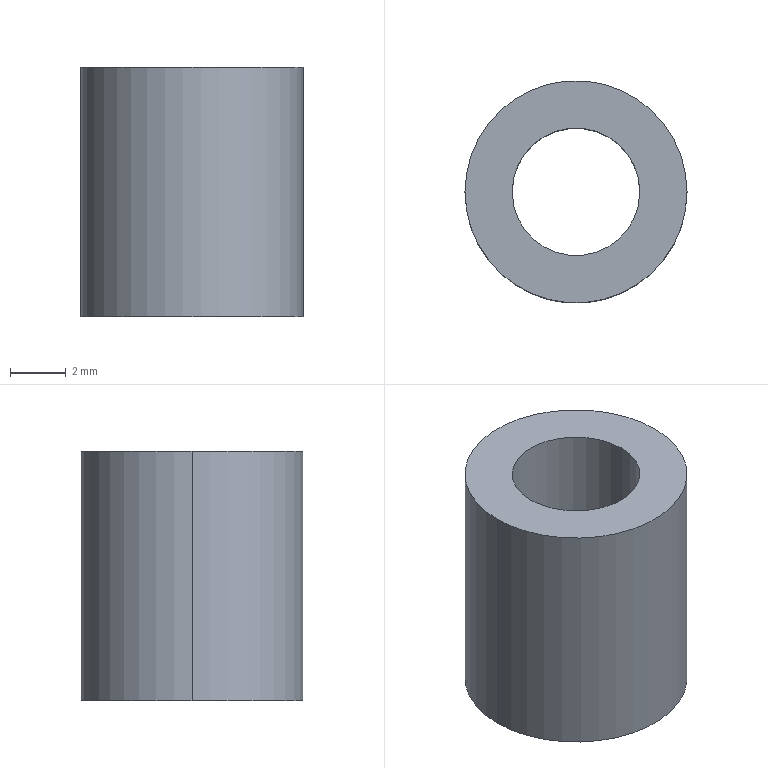Part | SolidWorks | features Extrusion 1 | 1 solid | 6 faces | box 8 x 8 x 9 mm | volume 302.818 mm3 | cylinder 4 | plane 2 | commonest cylinder face diameters 4.6 x2 8 x2
STEP:
#1=CARTESIAN_POINT('',(-2.3,0.,9.));
#2=VERTEX_POINT('',#1);
#3=CARTESIAN_POINT('',(2.3,0.,9.));
#4=VERTEX_POINT('',#3);
#5=CARTESIAN_POINT('',(0.,0.,9.));
#6=DIRECTION('',(0.,0.,1.));
#7=DIRECTION('',(1.,0.,0.));
#8=AXIS2_PLACEMENT_3D('',#5,#6,#7);
#9=CIRCLE('',#8,2.3);
#10=EDGE_CURVE('',#2,#4,#9,.T.);
#11=ORIENTED_EDGE('',*,*,#10,.T.);
#12=CARTESIAN_POINT('',(2.3,0.,0.));
#13=VERTEX_POINT('',#12);
#14=CARTESIAN_POINT('',(2.3,0.,9.));
#15=DIRECTION('',(0.,0.,-1.));
#16=VECTOR('',#15,1000.);
#17=LINE('',#14,#16);
#18=EDGE_CURVE('',#4,#13,#17,.T.);
#19=ORIENTED_EDGE('',*,*,#18,.T.);
#20=CARTESIAN_POINT('',(-2.3,0.,0.));
#21=VERTEX_POINT('',#20);
#22=CARTESIAN_POINT('',(0.,0.,0.));
#23=DIRECTION('',(0.,0.,1.));
#24=DIRECTION('',(1.,0.,0.));
#25=AXIS2_PLACEMENT_3D('',#22,#23,#24);
#26=CIRCLE('',#25,2.3);
#27=EDGE_CURVE('',#21,#13,#26,.T.);
#28=ORIENTED_EDGE('',*,*,#27,.F.);
#29=CARTESIAN_POINT('',(-2.3,0.,9.));
#30=DIRECTION('',(0.,0.,-1.));
#31=VECTOR('',#30,1000.);
#32=LINE('',#29,#31);
#33=EDGE_CURVE('',#2,#21,#32,.T.);
#34=ORIENTED_EDGE('',*,*,#33,.F.);
#35=EDGE_LOOP('',(#11,#19,#28,#34));
#36=FACE_OUTER_BOUND('',#35,.T.);
#37=CARTESIAN_POINT('',(0.,0.,9.));
#38=DIRECTION('',(0.,0.,-1.));
#39=DIRECTION('',(-1.,0.,0.));
#40=AXIS2_PLACEMENT_3D('',#37,#38,#39);
#41=CYLINDRICAL_SURFACE('',#40,2.3);
#42=ADVANCED_FACE('',(#36),#41,.F.);
#43=CARTESIAN_POINT('',(4.,0.,9.));
#44=VERTEX_POINT('',#43);
#45=CARTESIAN_POINT('',(-4.,0.,9.));
#46=VERTEX_POINT('',#45);
#47=CARTESIAN_POINT('',(0.,0.,9.));
#48=DIRECTION('',(0.,0.,1.));
#49=DIRECTION('',(1.,0.,0.));
#50=AXIS2_PLACEMENT_3D('',#47,#48,#49);
#51=CIRCLE('',#50,4.);
#52=EDGE_CURVE('',#44,#46,#51,.T.);
#53=ORIENTED_EDGE('',*,*,#52,.F.);
#54=CARTESIAN_POINT('',(4.,0.,0.));
#55=VERTEX_POINT('',#54);
#56=CARTESIAN_POINT('',(4.,0.,9.));
#57=DIRECTION('',(0.,0.,-1.));
#58=VECTOR('',#57,1000.);
#59=LINE('',#56,#58);
#60=EDGE_CURVE('',#44,#55,#59,.T.);
#61=ORIENTED_EDGE('',*,*,#60,.T.);
#62=CARTESIAN_POINT('',(-4.,0.,0.));
#63=VERTEX_POINT('',#62);
#64=CARTESIAN_POINT('',(0.,0.,0.));
#65=DIRECTION('',(0.,0.,1.));
#66=DIRECTION('',(1.,0.,0.));
#67=AXIS2_PLACEMENT_3D('',#64,#65,#66);
#68=CIRCLE('',#67,4.);
#69=EDGE_CURVE('',#55,#63,#68,.T.);
#70=ORIENTED_EDGE('',*,*,#69,.T.);
#71=CARTESIAN_POINT('',(-4.,0.,9.));
#72=DIRECTION('',(0.,0.,-1.));
#73=VECTOR('',#72,1000.);
#74=LINE('',#71,#73);
#75=EDGE_CURVE('',#46,#63,#74,.T.);
#76=ORIENTED_EDGE('',*,*,#75,.F.);
#77=EDGE_LOOP('',(#53,#61,#70,#76));
#78=FACE_OUTER_BOUND('',#77,.T.);
#79=CARTESIAN_POINT('',(0.,0.,9.));
#80=DIRECTION('',(0.,0.,-1.));
#81=DIRECTION('',(-1.,0.,0.));
#82=AXIS2_PLACEMENT_3D('',#79,#80,#81);
#83=CYLINDRICAL_SURFACE('',#82,4.);
#84=ADVANCED_FACE('',(#78),#83,.T.);
#85=CARTESIAN_POINT('',(0.,0.,9.));
#86=DIRECTION('',(0.,0.,1.));
#87=DIRECTION('',(1.,0.,0.));
#88=AXIS2_PLACEMENT_3D('',#85,#86,#87);
#89=CIRCLE('',#88,4.);
#90=EDGE_CURVE('',#46,#44,#89,.T.);
#91=ORIENTED_EDGE('',*,*,#90,.T.);
#92=ORIENTED_EDGE('',*,*,#52,.T.);
#93=EDGE_LOOP('',(#91,#92));
#94=FACE_OUTER_BOUND('',#93,.T.);
#95=ORIENTED_EDGE('',*,*,#10,.F.);
#96=CARTESIAN_POINT('',(0.,0.,9.));
#97=DIRECTION('',(0.,0.,1.));
#98=DIRECTION('',(1.,0.,0.));
#99=AXIS2_PLACEMENT_3D('',#96,#97,#98);
#100=CIRCLE('',#99,2.3);
#101=EDGE_CURVE('',#4,#2,#100,.T.);
#102=ORIENTED_EDGE('',*,*,#101,.F.);
#103=EDGE_LOOP('',(#95,#102));
#104=FACE_BOUND('',#103,.T.);
#105=CARTESIAN_POINT('',(0.,0.,9.));
#106=DIRECTION('',(0.,0.,1.));
#107=DIRECTION('',(1.,0.,0.));
#108=AXIS2_PLACEMENT_3D('',#105,#106,#107);
#109=PLANE('',#108);
#110=ADVANCED_FACE('',(#94,#104),#109,.T.);
#111=CARTESIAN_POINT('',(0.,0.,0.));
#112=DIRECTION('',(0.,0.,1.));
#113=DIRECTION('',(1.,0.,0.));
#114=AXIS2_PLACEMENT_3D('',#111,#112,#113);
#115=CIRCLE('',#114,4.);
#116=EDGE_CURVE('',#63,#55,#115,.T.);
#117=ORIENTED_EDGE('',*,*,#116,.F.);
#118=ORIENTED_EDGE('',*,*,#69,.F.);
#119=EDGE_LOOP('',(#117,#118));
#120=FACE_OUTER_BOUND('',#119,.T.);
#121=ORIENTED_EDGE('',*,*,#27,.T.);
#122=CARTESIAN_POINT('',(0.,0.,0.));
#123=DIRECTION('',(0.,0.,1.));
#124=DIRECTION('',(1.,0.,0.));
#125=AXIS2_PLACEMENT_3D('',#122,#123,#124);
#126=CIRCLE('',#125,2.3);
#127=EDGE_CURVE('',#13,#21,#126,.T.);
#128=ORIENTED_EDGE('',*,*,#127,.T.);
#129=EDGE_LOOP('',(#121,#128));
#130=FACE_BOUND('',#129,.T.);
#131=CARTESIAN_POINT('',(0.,0.,0.));
#132=DIRECTION('',(0.,0.,1.));
#133=DIRECTION('',(1.,0.,0.));
#134=AXIS2_PLACEMENT_3D('',#131,#132,#133);
#135=PLANE('',#134);
#136=ADVANCED_FACE('',(#120,#130),#135,.F.);
#137=ORIENTED_EDGE('',*,*,#60,.F.);
#138=ORIENTED_EDGE('',*,*,#90,.F.);
#139=ORIENTED_EDGE('',*,*,#75,.T.);
#140=ORIENTED_EDGE('',*,*,#116,.T.);
#141=EDGE_LOOP('',(#137,#138,#139,#140));
#142=FACE_OUTER_BOUND('',#141,.T.);
#143=CARTESIAN_POINT('',(0.,0.,9.));
#144=DIRECTION('',(0.,0.,-1.));
#145=DIRECTION('',(-1.,0.,0.));
#146=AXIS2_PLACEMENT_3D('',#143,#144,#145);
#147=CYLINDRICAL_SURFACE('',#146,4.);
#148=ADVANCED_FACE('',(#142),#147,.T.);
#149=ORIENTED_EDGE('',*,*,#18,.F.);
#150=ORIENTED_EDGE('',*,*,#101,.T.);
#151=ORIENTED_EDGE('',*,*,#33,.T.);
#152=ORIENTED_EDGE('',*,*,#127,.F.);
#153=EDGE_LOOP('',(#149,#150,#151,#152));
#154=FACE_OUTER_BOUND('',#153,.T.);
#155=CARTESIAN_POINT('',(0.,0.,9.));
#156=DIRECTION('',(0.,0.,-1.));
#157=DIRECTION('',(-1.,0.,0.));
#158=AXIS2_PLACEMENT_3D('',#155,#156,#157);
#159=CYLINDRICAL_SURFACE('',#158,2.3);
#160=ADVANCED_FACE('',(#154),#159,.F.);
#161=CLOSED_SHELL('',(#42,#84,#110,#136,#148,#160));
#162=MANIFOLD_SOLID_BREP('',#161);
#163=CARTESIAN_POINT('',(0.,0.,0.));
#164=DIRECTION('',(0.,0.,1.));
#165=DIRECTION('',(1.,0.,0.));
#166=AXIS2_PLACEMENT_3D('',#163,#164,#165);
#167=(LENGTH_UNIT()NAMED_UNIT(*)SI_UNIT(.MILLI.,.METRE.));
#168=UNCERTAINTY_MEASURE_WITH_UNIT(LENGTH_MEASURE(0.00001),#167,'','');
#169=(NAMED_UNIT(*)PLANE_ANGLE_UNIT()SI_UNIT($,.RADIAN.));
#170=(NAMED_UNIT(*)SI_UNIT($,.STERADIAN.)SOLID_ANGLE_UNIT());
#171=(GEOMETRIC_REPRESENTATION_CONTEXT(3)GLOBAL_UNCERTAINTY_ASSIGNED_CONTEXT((#168))GLOBAL_UNIT_ASSIGNED_CONTEXT((#167,#169,#170))REPRESENTATION_CONTEXT('',''));
#172=ADVANCED_BREP_SHAPE_REPRESENTATION('',(#162,#166),#171);